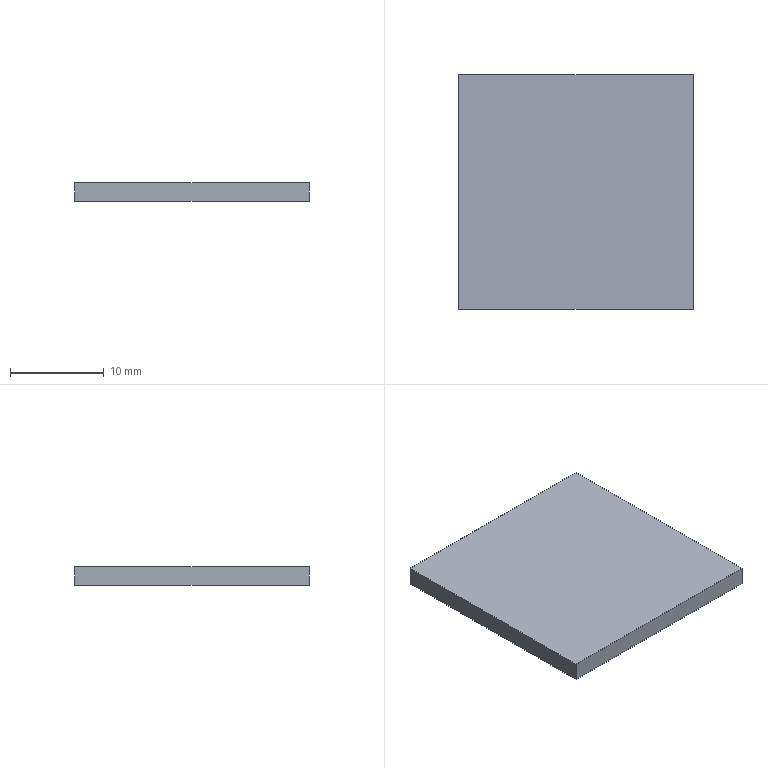Part | STEP file | Q7C1204 | 1 solid | 6 faces | box 25 x 25 x 2 mm | volume 1250 mm3 | plane 6
STEP:
#1=CARTESIAN_POINT('',(0.,0.,0.));
#2=DIRECTION('',(0.,0.,1.));
#3=DIRECTION('',(1.,0.,0.));
#4=AXIS2_PLACEMENT_3D('',#1,#2,#3);
#5=CARTESIAN_POINT('',(12.5,-12.5,0.));
#6=VERTEX_POINT('',#5);
#7=CARTESIAN_POINT('',(12.5,12.5,0.));
#8=VERTEX_POINT('',#7);
#9=CARTESIAN_POINT('',(12.5,12.5,0.));
#10=DIRECTION('',(0.,1.,0.));
#11=VECTOR('',#10,1.);
#12=LINE('',#9,#11);
#13=CARTESIAN_POINT('',(12.5,12.5,2.));
#14=DIRECTION('',(-1.,0.,0.));
#15=DIRECTION('',(0.,-1.,0.));
#16=AXIS2_PLACEMENT_3D('',#13,#14,#15);
#17=PLANE('',#16);
#18=CARTESIAN_POINT('',(0.,-2.));
#19=DIRECTION('',(-1.,0.));
#20=VECTOR('',#19,1.);
#21=LINE('',#18,#20);
#22=(GEOMETRIC_REPRESENTATION_CONTEXT(2)PARAMETRIC_REPRESENTATION_CONTEXT()REPRESENTATION_CONTEXT('',''));
#23=DEFINITIONAL_REPRESENTATION('',(#21),#22);
#24=PCURVE('',#17,#23);
#25=CARTESIAN_POINT('',(12.5,-12.5,0.));
#26=DIRECTION('',(0.,0.,1.));
#27=DIRECTION('',(1.,0.,0.));
#28=AXIS2_PLACEMENT_3D('',#25,#26,#27);
#29=PLANE('',#28);
#30=CARTESIAN_POINT('',(0.,25.));
#31=DIRECTION('',(0.,1.));
#32=VECTOR('',#31,1.);
#33=LINE('',#30,#32);
#34=(GEOMETRIC_REPRESENTATION_CONTEXT(2)PARAMETRIC_REPRESENTATION_CONTEXT()REPRESENTATION_CONTEXT('',''));
#35=DEFINITIONAL_REPRESENTATION('',(#33),#34);
#36=PCURVE('',#29,#35);
#37=SURFACE_CURVE('',#12,(#24,#36),.PCURVE_S1.);
#38=EDGE_CURVE('',#6,#8,#37,.T.);
#39=ORIENTED_EDGE('',*,*,#38,.T.);
#40=CARTESIAN_POINT('',(12.5,12.5,2.));
#41=VERTEX_POINT('',#40);
#42=CARTESIAN_POINT('',(12.5,12.5,2.));
#43=DIRECTION('',(0.,0.,-1.));
#44=VECTOR('',#43,1.);
#45=LINE('',#42,#44);
#46=CARTESIAN_POINT('',(0.,0.));
#47=DIRECTION('',(0.,-1.));
#48=VECTOR('',#47,1.);
#49=LINE('',#46,#48);
#50=(GEOMETRIC_REPRESENTATION_CONTEXT(2)PARAMETRIC_REPRESENTATION_CONTEXT()REPRESENTATION_CONTEXT('',''));
#51=DEFINITIONAL_REPRESENTATION('',(#49),#50);
#52=PCURVE('',#17,#51);
#53=CARTESIAN_POINT('',(12.5,12.5,2.));
#54=DIRECTION('',(0.,-1.,0.));
#55=DIRECTION('',(0.,0.,-1.));
#56=AXIS2_PLACEMENT_3D('',#53,#54,#55);
#57=PLANE('',#56);
#58=CARTESIAN_POINT('',(0.,0.));
#59=DIRECTION('',(1.,0.));
#60=VECTOR('',#59,1.);
#61=LINE('',#58,#60);
#62=(GEOMETRIC_REPRESENTATION_CONTEXT(2)PARAMETRIC_REPRESENTATION_CONTEXT()REPRESENTATION_CONTEXT('',''));
#63=DEFINITIONAL_REPRESENTATION('',(#61),#62);
#64=PCURVE('',#57,#63);
#65=SURFACE_CURVE('',#45,(#52,#64),.PCURVE_S1.);
#66=EDGE_CURVE('',#41,#8,#65,.T.);
#67=ORIENTED_EDGE('',*,*,#66,.F.);
#68=CARTESIAN_POINT('',(12.5,-12.5,2.));
#69=VERTEX_POINT('',#68);
#70=CARTESIAN_POINT('',(12.5,12.5,2.));
#71=DIRECTION('',(0.,1.,0.));
#72=VECTOR('',#71,1.);
#73=LINE('',#70,#72);
#74=CARTESIAN_POINT('',(0.,0.));
#75=DIRECTION('',(-1.,0.));
#76=VECTOR('',#75,1.);
#77=LINE('',#74,#76);
#78=(GEOMETRIC_REPRESENTATION_CONTEXT(2)PARAMETRIC_REPRESENTATION_CONTEXT()REPRESENTATION_CONTEXT('',''));
#79=DEFINITIONAL_REPRESENTATION('',(#77),#78);
#80=PCURVE('',#17,#79);
#81=CARTESIAN_POINT('',(12.5,-12.5,2.));
#82=DIRECTION('',(0.,0.,1.));
#83=DIRECTION('',(1.,0.,0.));
#84=AXIS2_PLACEMENT_3D('',#81,#82,#83);
#85=PLANE('',#84);
#86=CARTESIAN_POINT('',(0.,25.));
#87=DIRECTION('',(0.,1.));
#88=VECTOR('',#87,1.);
#89=LINE('',#86,#88);
#90=(GEOMETRIC_REPRESENTATION_CONTEXT(2)PARAMETRIC_REPRESENTATION_CONTEXT()REPRESENTATION_CONTEXT('',''));
#91=DEFINITIONAL_REPRESENTATION('',(#89),#90);
#92=PCURVE('',#85,#91);
#93=SURFACE_CURVE('',#73,(#80,#92),.PCURVE_S1.);
#94=EDGE_CURVE('',#69,#41,#93,.T.);
#95=ORIENTED_EDGE('',*,*,#94,.F.);
#96=CARTESIAN_POINT('',(12.5,-12.5,2.));
#97=DIRECTION('',(0.,0.,-1.));
#98=VECTOR('',#97,1.);
#99=LINE('',#96,#98);
#100=CARTESIAN_POINT('',(25.,0.));
#101=DIRECTION('',(0.,-1.));
#102=VECTOR('',#101,1.);
#103=LINE('',#100,#102);
#104=(GEOMETRIC_REPRESENTATION_CONTEXT(2)PARAMETRIC_REPRESENTATION_CONTEXT()REPRESENTATION_CONTEXT('',''));
#105=DEFINITIONAL_REPRESENTATION('',(#103),#104);
#106=PCURVE('',#17,#105);
#107=CARTESIAN_POINT('',(-12.5,-12.5,2.));
#108=DIRECTION('',(0.,1.,0.));
#109=DIRECTION('',(-1.,0.,0.));
#110=AXIS2_PLACEMENT_3D('',#107,#108,#109);
#111=PLANE('',#110);
#112=CARTESIAN_POINT('',(-25.,0.));
#113=DIRECTION('',(0.,-1.));
#114=VECTOR('',#113,1.);
#115=LINE('',#112,#114);
#116=(GEOMETRIC_REPRESENTATION_CONTEXT(2)PARAMETRIC_REPRESENTATION_CONTEXT()REPRESENTATION_CONTEXT('',''));
#117=DEFINITIONAL_REPRESENTATION('',(#115),#116);
#118=PCURVE('',#111,#117);
#119=SURFACE_CURVE('',#99,(#106,#118),.PCURVE_S1.);
#120=EDGE_CURVE('',#69,#6,#119,.T.);
#121=ORIENTED_EDGE('',*,*,#120,.T.);
#122=EDGE_LOOP('',(#39,#67,#95,#121));
#123=FACE_BOUND('',#122,.T.);
#124=ADVANCED_FACE('',(#123),#17,.F.);
#125=CARTESIAN_POINT('',(-12.5,12.5,0.));
#126=VERTEX_POINT('',#125);
#127=CARTESIAN_POINT('',(12.5,12.5,0.));
#128=DIRECTION('',(-1.,0.,0.));
#129=VECTOR('',#128,1.);
#130=LINE('',#127,#129);
#131=CARTESIAN_POINT('',(2.,0.));
#132=DIRECTION('',(0.,-1.));
#133=VECTOR('',#132,1.);
#134=LINE('',#131,#133);
#135=(GEOMETRIC_REPRESENTATION_CONTEXT(2)PARAMETRIC_REPRESENTATION_CONTEXT()REPRESENTATION_CONTEXT('',''));
#136=DEFINITIONAL_REPRESENTATION('',(#134),#135);
#137=PCURVE('',#57,#136);
#138=CARTESIAN_POINT('',(0.,25.));
#139=DIRECTION('',(-1.,0.));
#140=VECTOR('',#139,1.);
#141=LINE('',#138,#140);
#142=(GEOMETRIC_REPRESENTATION_CONTEXT(2)PARAMETRIC_REPRESENTATION_CONTEXT()REPRESENTATION_CONTEXT('',''));
#143=DEFINITIONAL_REPRESENTATION('',(#141),#142);
#144=PCURVE('',#29,#143);
#145=SURFACE_CURVE('',#130,(#137,#144),.PCURVE_S1.);
#146=EDGE_CURVE('',#8,#126,#145,.T.);
#147=ORIENTED_EDGE('',*,*,#146,.T.);
#148=CARTESIAN_POINT('',(-12.5,12.5,2.));
#149=VERTEX_POINT('',#148);
#150=CARTESIAN_POINT('',(-12.5,12.5,2.));
#151=DIRECTION('',(0.,0.,-1.));
#152=VECTOR('',#151,1.);
#153=LINE('',#150,#152);
#154=CARTESIAN_POINT('',(0.,-25.));
#155=DIRECTION('',(1.,0.));
#156=VECTOR('',#155,1.);
#157=LINE('',#154,#156);
#158=(GEOMETRIC_REPRESENTATION_CONTEXT(2)PARAMETRIC_REPRESENTATION_CONTEXT()REPRESENTATION_CONTEXT('',''));
#159=DEFINITIONAL_REPRESENTATION('',(#157),#158);
#160=PCURVE('',#57,#159);
#161=CARTESIAN_POINT('',(-12.5,12.5,2.));
#162=DIRECTION('',(1.,0.,0.));
#163=DIRECTION('',(0.,1.,0.));
#164=AXIS2_PLACEMENT_3D('',#161,#162,#163);
#165=PLANE('',#164);
#166=CARTESIAN_POINT('',(0.,0.));
#167=DIRECTION('',(0.,-1.));
#168=VECTOR('',#167,1.);
#169=LINE('',#166,#168);
#170=(GEOMETRIC_REPRESENTATION_CONTEXT(2)PARAMETRIC_REPRESENTATION_CONTEXT()REPRESENTATION_CONTEXT('',''));
#171=DEFINITIONAL_REPRESENTATION('',(#169),#170);
#172=PCURVE('',#165,#171);
#173=SURFACE_CURVE('',#153,(#160,#172),.PCURVE_S1.);
#174=EDGE_CURVE('',#149,#126,#173,.T.);
#175=ORIENTED_EDGE('',*,*,#174,.F.);
#176=CARTESIAN_POINT('',(12.5,12.5,2.));
#177=DIRECTION('',(-1.,0.,0.));
#178=VECTOR('',#177,1.);
#179=LINE('',#176,#178);
#180=CARTESIAN_POINT('',(0.,0.));
#181=DIRECTION('',(0.,-1.));
#182=VECTOR('',#181,1.);
#183=LINE('',#180,#182);
#184=(GEOMETRIC_REPRESENTATION_CONTEXT(2)PARAMETRIC_REPRESENTATION_CONTEXT()REPRESENTATION_CONTEXT('',''));
#185=DEFINITIONAL_REPRESENTATION('',(#183),#184);
#186=PCURVE('',#57,#185);
#187=CARTESIAN_POINT('',(0.,25.));
#188=DIRECTION('',(-1.,0.));
#189=VECTOR('',#188,1.);
#190=LINE('',#187,#189);
#191=(GEOMETRIC_REPRESENTATION_CONTEXT(2)PARAMETRIC_REPRESENTATION_CONTEXT()REPRESENTATION_CONTEXT('',''));
#192=DEFINITIONAL_REPRESENTATION('',(#190),#191);
#193=PCURVE('',#85,#192);
#194=SURFACE_CURVE('',#179,(#186,#193),.PCURVE_S1.);
#195=EDGE_CURVE('',#41,#149,#194,.T.);
#196=ORIENTED_EDGE('',*,*,#195,.F.);
#197=ORIENTED_EDGE('',*,*,#66,.T.);
#198=EDGE_LOOP('',(#147,#175,#196,#197));
#199=FACE_BOUND('',#198,.T.);
#200=ADVANCED_FACE('',(#199),#57,.F.);
#201=CARTESIAN_POINT('',(-12.5,-12.5,0.));
#202=VERTEX_POINT('',#201);
#203=CARTESIAN_POINT('',(-12.5,12.5,0.));
#204=DIRECTION('',(0.,-1.,0.));
#205=VECTOR('',#204,1.);
#206=LINE('',#203,#205);
#207=CARTESIAN_POINT('',(0.,-2.));
#208=DIRECTION('',(-1.,0.));
#209=VECTOR('',#208,1.);
#210=LINE('',#207,#209);
#211=(GEOMETRIC_REPRESENTATION_CONTEXT(2)PARAMETRIC_REPRESENTATION_CONTEXT()REPRESENTATION_CONTEXT('',''));
#212=DEFINITIONAL_REPRESENTATION('',(#210),#211);
#213=PCURVE('',#165,#212);
#214=CARTESIAN_POINT('',(-25.,25.));
#215=DIRECTION('',(0.,-1.));
#216=VECTOR('',#215,1.);
#217=LINE('',#214,#216);
#218=(GEOMETRIC_REPRESENTATION_CONTEXT(2)PARAMETRIC_REPRESENTATION_CONTEXT()REPRESENTATION_CONTEXT('',''));
#219=DEFINITIONAL_REPRESENTATION('',(#217),#218);
#220=PCURVE('',#29,#219);
#221=SURFACE_CURVE('',#206,(#213,#220),.PCURVE_S1.);
#222=EDGE_CURVE('',#126,#202,#221,.T.);
#223=ORIENTED_EDGE('',*,*,#222,.T.);
#224=CARTESIAN_POINT('',(-12.5,-12.5,2.));
#225=VERTEX_POINT('',#224);
#226=CARTESIAN_POINT('',(-12.5,-12.5,2.));
#227=DIRECTION('',(0.,0.,-1.));
#228=VECTOR('',#227,1.);
#229=LINE('',#226,#228);
#230=CARTESIAN_POINT('',(-25.,0.));
#231=DIRECTION('',(0.,-1.));
#232=VECTOR('',#231,1.);
#233=LINE('',#230,#232);
#234=(GEOMETRIC_REPRESENTATION_CONTEXT(2)PARAMETRIC_REPRESENTATION_CONTEXT()REPRESENTATION_CONTEXT('',''));
#235=DEFINITIONAL_REPRESENTATION('',(#233),#234);
#236=PCURVE('',#165,#235);
#237=CARTESIAN_POINT('',(0.,0.));
#238=DIRECTION('',(0.,-1.));
#239=VECTOR('',#238,1.);
#240=LINE('',#237,#239);
#241=(GEOMETRIC_REPRESENTATION_CONTEXT(2)PARAMETRIC_REPRESENTATION_CONTEXT()REPRESENTATION_CONTEXT('',''));
#242=DEFINITIONAL_REPRESENTATION('',(#240),#241);
#243=PCURVE('',#111,#242);
#244=SURFACE_CURVE('',#229,(#236,#243),.PCURVE_S1.);
#245=EDGE_CURVE('',#225,#202,#244,.T.);
#246=ORIENTED_EDGE('',*,*,#245,.F.);
#247=CARTESIAN_POINT('',(-12.5,12.5,2.));
#248=DIRECTION('',(0.,-1.,0.));
#249=VECTOR('',#248,1.);
#250=LINE('',#247,#249);
#251=CARTESIAN_POINT('',(0.,0.));
#252=DIRECTION('',(-1.,0.));
#253=VECTOR('',#252,1.);
#254=LINE('',#251,#253);
#255=(GEOMETRIC_REPRESENTATION_CONTEXT(2)PARAMETRIC_REPRESENTATION_CONTEXT()REPRESENTATION_CONTEXT('',''));
#256=DEFINITIONAL_REPRESENTATION('',(#254),#255);
#257=PCURVE('',#165,#256);
#258=CARTESIAN_POINT('',(-25.,25.));
#259=DIRECTION('',(0.,-1.));
#260=VECTOR('',#259,1.);
#261=LINE('',#258,#260);
#262=(GEOMETRIC_REPRESENTATION_CONTEXT(2)PARAMETRIC_REPRESENTATION_CONTEXT()REPRESENTATION_CONTEXT('',''));
#263=DEFINITIONAL_REPRESENTATION('',(#261),#262);
#264=PCURVE('',#85,#263);
#265=SURFACE_CURVE('',#250,(#257,#264),.PCURVE_S1.);
#266=EDGE_CURVE('',#149,#225,#265,.T.);
#267=ORIENTED_EDGE('',*,*,#266,.F.);
#268=ORIENTED_EDGE('',*,*,#174,.T.);
#269=EDGE_LOOP('',(#223,#246,#267,#268));
#270=FACE_BOUND('',#269,.T.);
#271=ADVANCED_FACE('',(#270),#165,.F.);
#272=CARTESIAN_POINT('',(-12.5,-12.5,0.));
#273=DIRECTION('',(1.,0.,0.));
#274=VECTOR('',#273,1.);
#275=LINE('',#272,#274);
#276=CARTESIAN_POINT('',(0.,-2.));
#277=DIRECTION('',(-1.,0.));
#278=VECTOR('',#277,1.);
#279=LINE('',#276,#278);
#280=(GEOMETRIC_REPRESENTATION_CONTEXT(2)PARAMETRIC_REPRESENTATION_CONTEXT()REPRESENTATION_CONTEXT('',''));
#281=DEFINITIONAL_REPRESENTATION('',(#279),#280);
#282=PCURVE('',#111,#281);
#283=CARTESIAN_POINT('',(-25.,0.));
#284=DIRECTION('',(1.,0.));
#285=VECTOR('',#284,1.);
#286=LINE('',#283,#285);
#287=(GEOMETRIC_REPRESENTATION_CONTEXT(2)PARAMETRIC_REPRESENTATION_CONTEXT()REPRESENTATION_CONTEXT('',''));
#288=DEFINITIONAL_REPRESENTATION('',(#286),#287);
#289=PCURVE('',#29,#288);
#290=SURFACE_CURVE('',#275,(#282,#289),.PCURVE_S1.);
#291=EDGE_CURVE('',#202,#6,#290,.T.);
#292=ORIENTED_EDGE('',*,*,#291,.T.);
#293=ORIENTED_EDGE('',*,*,#120,.F.);
#294=CARTESIAN_POINT('',(-12.5,-12.5,2.));
#295=DIRECTION('',(1.,0.,0.));
#296=VECTOR('',#295,1.);
#297=LINE('',#294,#296);
#298=CARTESIAN_POINT('',(0.,0.));
#299=DIRECTION('',(-1.,0.));
#300=VECTOR('',#299,1.);
#301=LINE('',#298,#300);
#302=(GEOMETRIC_REPRESENTATION_CONTEXT(2)PARAMETRIC_REPRESENTATION_CONTEXT()REPRESENTATION_CONTEXT('',''));
#303=DEFINITIONAL_REPRESENTATION('',(#301),#302);
#304=PCURVE('',#111,#303);
#305=CARTESIAN_POINT('',(-25.,0.));
#306=DIRECTION('',(1.,0.));
#307=VECTOR('',#306,1.);
#308=LINE('',#305,#307);
#309=(GEOMETRIC_REPRESENTATION_CONTEXT(2)PARAMETRIC_REPRESENTATION_CONTEXT()REPRESENTATION_CONTEXT('',''));
#310=DEFINITIONAL_REPRESENTATION('',(#308),#309);
#311=PCURVE('',#85,#310);
#312=SURFACE_CURVE('',#297,(#304,#311),.PCURVE_S1.);
#313=EDGE_CURVE('',#225,#69,#312,.T.);
#314=ORIENTED_EDGE('',*,*,#313,.F.);
#315=ORIENTED_EDGE('',*,*,#245,.T.);
#316=EDGE_LOOP('',(#292,#293,#314,#315));
#317=FACE_BOUND('',#316,.T.);
#318=ADVANCED_FACE('',(#317),#111,.F.);
#319=ORIENTED_EDGE('',*,*,#94,.T.);
#320=ORIENTED_EDGE('',*,*,#195,.T.);
#321=ORIENTED_EDGE('',*,*,#266,.T.);
#322=ORIENTED_EDGE('',*,*,#313,.T.);
#323=EDGE_LOOP('',(#319,#320,#321,#322));
#324=FACE_BOUND('',#323,.T.);
#325=ADVANCED_FACE('',(#324),#85,.T.);
#326=ORIENTED_EDGE('',*,*,#38,.F.);
#327=ORIENTED_EDGE('',*,*,#291,.F.);
#328=ORIENTED_EDGE('',*,*,#222,.F.);
#329=ORIENTED_EDGE('',*,*,#146,.F.);
#330=EDGE_LOOP('',(#326,#327,#328,#329));
#331=FACE_BOUND('',#330,.T.);
#332=ADVANCED_FACE('',(#331),#29,.F.);
#333=CLOSED_SHELL('',(#124,#200,#271,#318,#325,#332));
#334=MANIFOLD_SOLID_BREP('',#333);
#335=(LENGTH_UNIT()NAMED_UNIT(*)SI_UNIT(.MILLI.,.METRE.));
#336=UNCERTAINTY_MEASURE_WITH_UNIT(LENGTH_MEASURE(0.0000001),#335,'','');
#337=(NAMED_UNIT(*)PLANE_ANGLE_UNIT()SI_UNIT($,.RADIAN.));
#338=(NAMED_UNIT(*)SI_UNIT($,.STERADIAN.)SOLID_ANGLE_UNIT());
#339=(GEOMETRIC_REPRESENTATION_CONTEXT(3)GLOBAL_UNCERTAINTY_ASSIGNED_CONTEXT((#336))GLOBAL_UNIT_ASSIGNED_CONTEXT((#335,#337,#338))REPRESENTATION_CONTEXT('',''));
#340=ADVANCED_BREP_SHAPE_REPRESENTATION('',(#4,#334),#339);